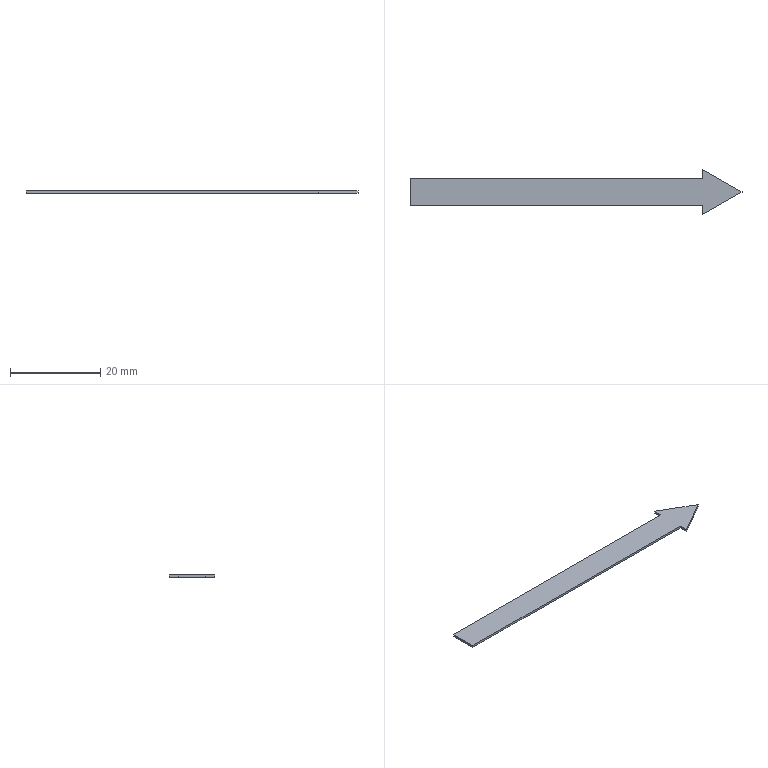Part | STEP file | [Flow direction nameplate]-Part-1 | 1 solid | 9 faces | box 73.66 x 10 x 0.5 mm | volume 216.651 mm3 | plane 9
STEP:
#1=CARTESIAN_POINT('',(-311.498,-34.081,51.35));
#2=VERTEX_POINT('',#1);
#3=CARTESIAN_POINT('',(-311.498,-40.081,51.35));
#4=VERTEX_POINT('',#3);
#5=CARTESIAN_POINT('',(-311.498,-34.081,51.35));
#6=DIRECTION('',(0.,-1.,0.));
#7=VECTOR('',#6,1000.);
#8=LINE('',#5,#7);
#9=EDGE_CURVE('',#2,#4,#8,.T.);
#10=ORIENTED_EDGE('',*,*,#9,.T.);
#11=CARTESIAN_POINT('',(-311.498,-40.081,51.85));
#12=VERTEX_POINT('',#11);
#13=CARTESIAN_POINT('',(-311.498,-40.081,51.85));
#14=DIRECTION('',(0.,0.,-1.));
#15=VECTOR('',#14,1000.);
#16=LINE('',#13,#15);
#17=EDGE_CURVE('',#12,#4,#16,.T.);
#18=ORIENTED_EDGE('',*,*,#17,.F.);
#19=CARTESIAN_POINT('',(-311.498,-34.081,51.85));
#20=VERTEX_POINT('',#19);
#21=CARTESIAN_POINT('',(-311.498,-34.081,51.85));
#22=DIRECTION('',(0.,-1.,0.));
#23=VECTOR('',#22,1000.);
#24=LINE('',#21,#23);
#25=EDGE_CURVE('',#20,#12,#24,.T.);
#26=ORIENTED_EDGE('',*,*,#25,.F.);
#27=CARTESIAN_POINT('',(-311.498,-34.081,51.85));
#28=DIRECTION('',(0.,0.,-1.));
#29=VECTOR('',#28,1000.);
#30=LINE('',#27,#29);
#31=EDGE_CURVE('',#20,#2,#30,.T.);
#32=ORIENTED_EDGE('',*,*,#31,.T.);
#33=EDGE_LOOP('',(#10,#18,#26,#32));
#34=FACE_OUTER_BOUND('',#33,.T.);
#35=CARTESIAN_POINT('',(-311.498,-34.081,51.85));
#36=DIRECTION('',(1.,0.,0.));
#37=DIRECTION('',(0.,0.,-1.));
#38=AXIS2_PLACEMENT_3D('',#35,#36,#37);
#39=PLANE('',#38);
#40=ADVANCED_FACE('',(#34),#39,.F.);
#41=CARTESIAN_POINT('',(-246.498,-40.081,51.35));
#42=VERTEX_POINT('',#41);
#43=CARTESIAN_POINT('',(-311.498,-40.081,51.35));
#44=DIRECTION('',(1.,0.,0.));
#45=VECTOR('',#44,1000.);
#46=LINE('',#43,#45);
#47=EDGE_CURVE('',#4,#42,#46,.T.);
#48=ORIENTED_EDGE('',*,*,#47,.T.);
#49=CARTESIAN_POINT('',(-246.498,-40.081,51.85));
#50=VERTEX_POINT('',#49);
#51=CARTESIAN_POINT('',(-246.498,-40.081,51.85));
#52=DIRECTION('',(0.,0.,-1.));
#53=VECTOR('',#52,1000.);
#54=LINE('',#51,#53);
#55=EDGE_CURVE('',#50,#42,#54,.T.);
#56=ORIENTED_EDGE('',*,*,#55,.F.);
#57=CARTESIAN_POINT('',(-311.498,-40.081,51.85));
#58=DIRECTION('',(1.,0.,0.));
#59=VECTOR('',#58,1000.);
#60=LINE('',#57,#59);
#61=EDGE_CURVE('',#12,#50,#60,.T.);
#62=ORIENTED_EDGE('',*,*,#61,.F.);
#63=ORIENTED_EDGE('',*,*,#17,.T.);
#64=EDGE_LOOP('',(#48,#56,#62,#63));
#65=FACE_OUTER_BOUND('',#64,.T.);
#66=CARTESIAN_POINT('',(-311.498,-40.081,51.85));
#67=DIRECTION('',(0.,1.,0.));
#68=DIRECTION('',(0.,0.,-1.));
#69=AXIS2_PLACEMENT_3D('',#66,#67,#68);
#70=PLANE('',#69);
#71=ADVANCED_FACE('',(#65),#70,.F.);
#72=CARTESIAN_POINT('',(-246.498,-42.081,51.35));
#73=VERTEX_POINT('',#72);
#74=CARTESIAN_POINT('',(-246.498,-40.081,51.35));
#75=DIRECTION('',(0.,-1.,0.));
#76=VECTOR('',#75,1000.);
#77=LINE('',#74,#76);
#78=EDGE_CURVE('',#42,#73,#77,.T.);
#79=ORIENTED_EDGE('',*,*,#78,.T.);
#80=CARTESIAN_POINT('',(-246.498,-42.081,51.85));
#81=VERTEX_POINT('',#80);
#82=CARTESIAN_POINT('',(-246.498,-42.081,51.85));
#83=DIRECTION('',(0.,0.,-1.));
#84=VECTOR('',#83,1000.);
#85=LINE('',#82,#84);
#86=EDGE_CURVE('',#81,#73,#85,.T.);
#87=ORIENTED_EDGE('',*,*,#86,.F.);
#88=CARTESIAN_POINT('',(-246.498,-40.081,51.85));
#89=DIRECTION('',(0.,-1.,0.));
#90=VECTOR('',#89,1000.);
#91=LINE('',#88,#90);
#92=EDGE_CURVE('',#50,#81,#91,.T.);
#93=ORIENTED_EDGE('',*,*,#92,.F.);
#94=ORIENTED_EDGE('',*,*,#55,.T.);
#95=EDGE_LOOP('',(#79,#87,#93,#94));
#96=FACE_OUTER_BOUND('',#95,.T.);
#97=CARTESIAN_POINT('',(-246.498,-40.081,51.85));
#98=DIRECTION('',(1.,0.,0.));
#99=DIRECTION('',(0.,0.,-1.));
#100=AXIS2_PLACEMENT_3D('',#97,#98,#99);
#101=PLANE('',#100);
#102=ADVANCED_FACE('',(#96),#101,.F.);
#103=CARTESIAN_POINT('',(-237.838,-37.081,51.35));
#104=VERTEX_POINT('',#103);
#105=CARTESIAN_POINT('',(-246.498,-42.081,51.35));
#106=DIRECTION('',(0.866,0.5,0.));
#107=VECTOR('',#106,1000.);
#108=LINE('',#105,#107);
#109=EDGE_CURVE('',#73,#104,#108,.T.);
#110=ORIENTED_EDGE('',*,*,#109,.T.);
#111=CARTESIAN_POINT('',(-237.838,-37.081,51.85));
#112=VERTEX_POINT('',#111);
#113=CARTESIAN_POINT('',(-237.838,-37.081,51.85));
#114=DIRECTION('',(0.,0.,-1.));
#115=VECTOR('',#114,1000.);
#116=LINE('',#113,#115);
#117=EDGE_CURVE('',#112,#104,#116,.T.);
#118=ORIENTED_EDGE('',*,*,#117,.F.);
#119=CARTESIAN_POINT('',(-246.498,-42.081,51.85));
#120=DIRECTION('',(0.866,0.5,0.));
#121=VECTOR('',#120,1000.);
#122=LINE('',#119,#121);
#123=EDGE_CURVE('',#81,#112,#122,.T.);
#124=ORIENTED_EDGE('',*,*,#123,.F.);
#125=ORIENTED_EDGE('',*,*,#86,.T.);
#126=EDGE_LOOP('',(#110,#118,#124,#125));
#127=FACE_OUTER_BOUND('',#126,.T.);
#128=CARTESIAN_POINT('',(-246.498,-42.081,51.85));
#129=DIRECTION('',(-0.5,0.866,0.));
#130=DIRECTION('',(-0.866,-0.5,0.));
#131=AXIS2_PLACEMENT_3D('',#128,#129,#130);
#132=PLANE('',#131);
#133=ADVANCED_FACE('',(#127),#132,.F.);
#134=CARTESIAN_POINT('',(-246.498,-32.081,51.35));
#135=VERTEX_POINT('',#134);
#136=CARTESIAN_POINT('',(-237.838,-37.081,51.35));
#137=DIRECTION('',(-0.866,0.5,0.));
#138=VECTOR('',#137,1000.);
#139=LINE('',#136,#138);
#140=EDGE_CURVE('',#104,#135,#139,.T.);
#141=ORIENTED_EDGE('',*,*,#140,.T.);
#142=CARTESIAN_POINT('',(-246.498,-32.081,51.85));
#143=VERTEX_POINT('',#142);
#144=CARTESIAN_POINT('',(-246.498,-32.081,51.85));
#145=DIRECTION('',(0.,0.,-1.));
#146=VECTOR('',#145,1000.);
#147=LINE('',#144,#146);
#148=EDGE_CURVE('',#143,#135,#147,.T.);
#149=ORIENTED_EDGE('',*,*,#148,.F.);
#150=CARTESIAN_POINT('',(-237.838,-37.081,51.85));
#151=DIRECTION('',(-0.866,0.5,0.));
#152=VECTOR('',#151,1000.);
#153=LINE('',#150,#152);
#154=EDGE_CURVE('',#112,#143,#153,.T.);
#155=ORIENTED_EDGE('',*,*,#154,.F.);
#156=ORIENTED_EDGE('',*,*,#117,.T.);
#157=EDGE_LOOP('',(#141,#149,#155,#156));
#158=FACE_OUTER_BOUND('',#157,.T.);
#159=CARTESIAN_POINT('',(-237.838,-37.081,51.85));
#160=DIRECTION('',(-0.5,-0.866,0.));
#161=DIRECTION('',(0.866,-0.5,0.));
#162=AXIS2_PLACEMENT_3D('',#159,#160,#161);
#163=PLANE('',#162);
#164=ADVANCED_FACE('',(#158),#163,.F.);
#165=CARTESIAN_POINT('',(-246.498,-34.081,51.35));
#166=VERTEX_POINT('',#165);
#167=CARTESIAN_POINT('',(-246.498,-32.081,51.35));
#168=DIRECTION('',(0.,-1.,0.));
#169=VECTOR('',#168,1000.);
#170=LINE('',#167,#169);
#171=EDGE_CURVE('',#135,#166,#170,.T.);
#172=ORIENTED_EDGE('',*,*,#171,.T.);
#173=CARTESIAN_POINT('',(-246.498,-34.081,51.85));
#174=VERTEX_POINT('',#173);
#175=CARTESIAN_POINT('',(-246.498,-34.081,51.85));
#176=DIRECTION('',(0.,0.,-1.));
#177=VECTOR('',#176,1000.);
#178=LINE('',#175,#177);
#179=EDGE_CURVE('',#174,#166,#178,.T.);
#180=ORIENTED_EDGE('',*,*,#179,.F.);
#181=CARTESIAN_POINT('',(-246.498,-32.081,51.85));
#182=DIRECTION('',(0.,-1.,0.));
#183=VECTOR('',#182,1000.);
#184=LINE('',#181,#183);
#185=EDGE_CURVE('',#143,#174,#184,.T.);
#186=ORIENTED_EDGE('',*,*,#185,.F.);
#187=ORIENTED_EDGE('',*,*,#148,.T.);
#188=EDGE_LOOP('',(#172,#180,#186,#187));
#189=FACE_OUTER_BOUND('',#188,.T.);
#190=CARTESIAN_POINT('',(-246.498,-32.081,51.85));
#191=DIRECTION('',(1.,0.,0.));
#192=DIRECTION('',(0.,0.,-1.));
#193=AXIS2_PLACEMENT_3D('',#190,#191,#192);
#194=PLANE('',#193);
#195=ADVANCED_FACE('',(#189),#194,.F.);
#196=CARTESIAN_POINT('',(-246.498,-34.081,51.35));
#197=DIRECTION('',(-1.,0.,0.));
#198=VECTOR('',#197,1000.);
#199=LINE('',#196,#198);
#200=EDGE_CURVE('',#166,#2,#199,.T.);
#201=ORIENTED_EDGE('',*,*,#200,.T.);
#202=ORIENTED_EDGE('',*,*,#31,.F.);
#203=CARTESIAN_POINT('',(-246.498,-34.081,51.85));
#204=DIRECTION('',(-1.,0.,0.));
#205=VECTOR('',#204,1000.);
#206=LINE('',#203,#205);
#207=EDGE_CURVE('',#174,#20,#206,.T.);
#208=ORIENTED_EDGE('',*,*,#207,.F.);
#209=ORIENTED_EDGE('',*,*,#179,.T.);
#210=EDGE_LOOP('',(#201,#202,#208,#209));
#211=FACE_OUTER_BOUND('',#210,.T.);
#212=CARTESIAN_POINT('',(-246.498,-34.081,51.85));
#213=DIRECTION('',(0.,-1.,0.));
#214=DIRECTION('',(0.,0.,1.));
#215=AXIS2_PLACEMENT_3D('',#212,#213,#214);
#216=PLANE('',#215);
#217=ADVANCED_FACE('',(#211),#216,.F.);
#218=ORIENTED_EDGE('',*,*,#25,.T.);
#219=ORIENTED_EDGE('',*,*,#61,.T.);
#220=ORIENTED_EDGE('',*,*,#92,.T.);
#221=ORIENTED_EDGE('',*,*,#123,.T.);
#222=ORIENTED_EDGE('',*,*,#154,.T.);
#223=ORIENTED_EDGE('',*,*,#185,.T.);
#224=ORIENTED_EDGE('',*,*,#207,.T.);
#225=EDGE_LOOP('',(#218,#219,#220,#221,#222,#223,#224));
#226=FACE_OUTER_BOUND('',#225,.T.);
#227=CARTESIAN_POINT('',(-270.381,-35.464,51.85));
#228=DIRECTION('',(0.,0.,1.));
#229=DIRECTION('',(0.,1.,0.));
#230=AXIS2_PLACEMENT_3D('',#227,#228,#229);
#231=PLANE('',#230);
#232=ADVANCED_FACE('',(#226),#231,.T.);
#233=ORIENTED_EDGE('',*,*,#9,.F.);
#234=ORIENTED_EDGE('',*,*,#200,.F.);
#235=ORIENTED_EDGE('',*,*,#171,.F.);
#236=ORIENTED_EDGE('',*,*,#140,.F.);
#237=ORIENTED_EDGE('',*,*,#109,.F.);
#238=ORIENTED_EDGE('',*,*,#78,.F.);
#239=ORIENTED_EDGE('',*,*,#47,.F.);
#240=EDGE_LOOP('',(#233,#234,#235,#236,#237,#238,#239));
#241=FACE_OUTER_BOUND('',#240,.T.);
#242=CARTESIAN_POINT('',(-270.381,-35.464,51.35));
#243=DIRECTION('',(0.,0.,1.));
#244=DIRECTION('',(0.,1.,0.));
#245=AXIS2_PLACEMENT_3D('',#242,#243,#244);
#246=PLANE('',#245);
#247=ADVANCED_FACE('',(#241),#246,.F.);
#248=CLOSED_SHELL('',(#40,#71,#102,#133,#164,#195,#217,#232,#247));
#249=MANIFOLD_SOLID_BREP('',#248);
#250=CARTESIAN_POINT('',(0.,0.,0.));
#251=DIRECTION('',(0.,0.,1.));
#252=DIRECTION('',(1.,0.,0.));
#253=AXIS2_PLACEMENT_3D('',#250,#251,#252);
#254=(LENGTH_UNIT()NAMED_UNIT(*)SI_UNIT(.MILLI.,.METRE.));
#255=UNCERTAINTY_MEASURE_WITH_UNIT(LENGTH_MEASURE(0.00001),#254,'','');
#256=(NAMED_UNIT(*)PLANE_ANGLE_UNIT()SI_UNIT($,.RADIAN.));
#257=(NAMED_UNIT(*)SI_UNIT($,.STERADIAN.)SOLID_ANGLE_UNIT());
#258=(GEOMETRIC_REPRESENTATION_CONTEXT(3)GLOBAL_UNCERTAINTY_ASSIGNED_CONTEXT((#255))GLOBAL_UNIT_ASSIGNED_CONTEXT((#254,#256,#257))REPRESENTATION_CONTEXT('',''));
#259=ADVANCED_BREP_SHAPE_REPRESENTATION('',(#249,#253),#258);